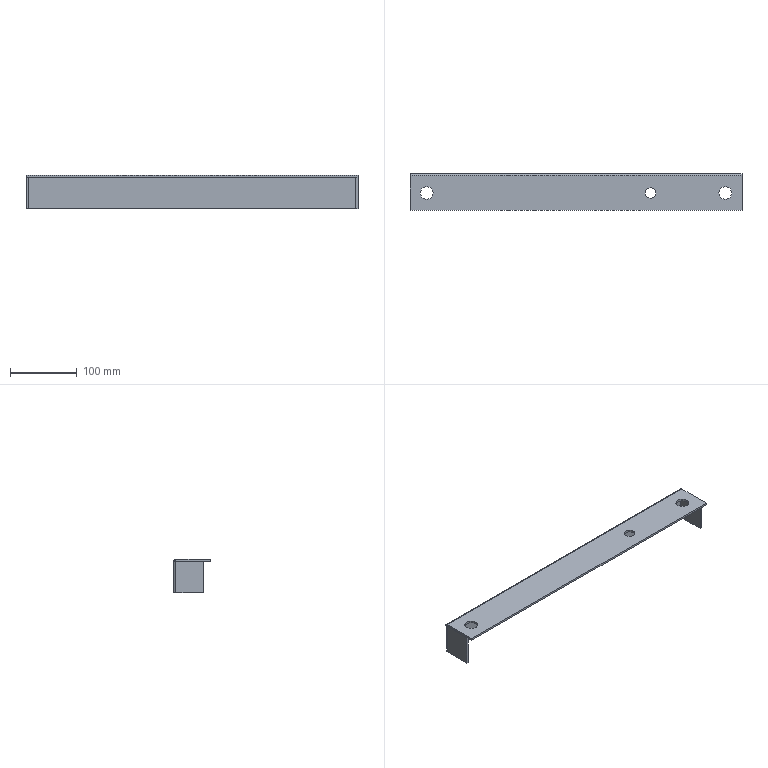Part | STEP file | 1 solid | 38 faces | box 498 x 55 x 50 mm | volume 160582 mm3 | plane 26 | cylinder 12 | commonest cylinder face diameters 19 x4 0.4 x3 6.4 x3 16 x2